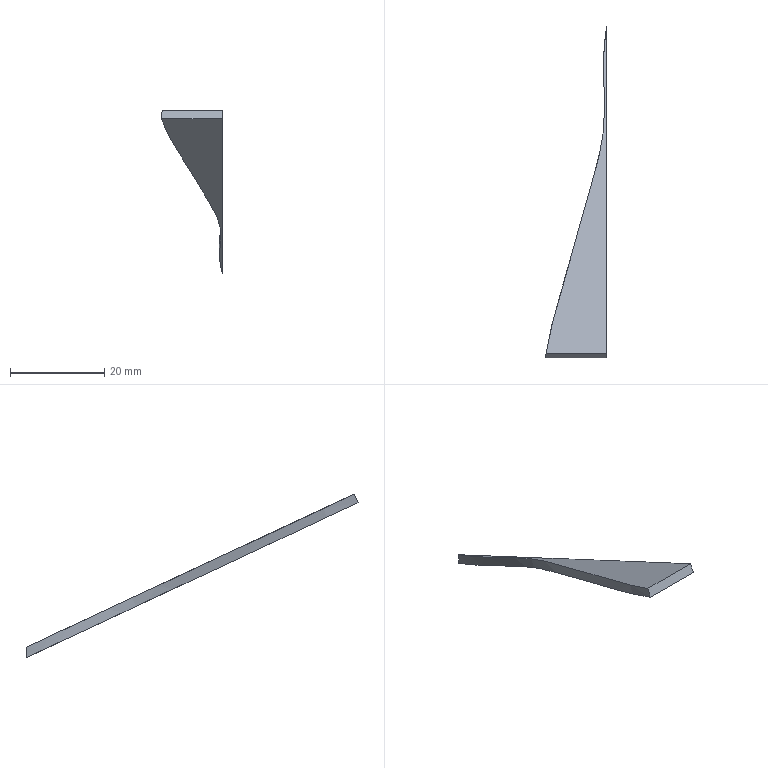Part | NX | features solid 2 | 1 solid | 5 faces | box 12.913 x 70.296 x 34.592 mm | volume 729.342 mm3 | plane 4 | spline 1
STEP:
#1=CARTESIAN_POINT('',(764.53,225.774,-99.063));
#2=VERTEX_POINT('',#1);
#3=CARTESIAN_POINT('',(777.317,295.224,-131.448));
#4=VERTEX_POINT('',#3);
#5=CARTESIAN_POINT('',(764.53,225.774,-99.063));
#6=CARTESIAN_POINT('',(764.988,228.719,-100.436));
#7=CARTESIAN_POINT('',(766.283,234.526,-103.144));
#8=CARTESIAN_POINT('',(768.978,243.072,-107.129));
#9=CARTESIAN_POINT('',(771.329,251.695,-111.15));
#10=CARTESIAN_POINT('',(773.684,260.31,-115.167));
#11=CARTESIAN_POINT('',(776.335,268.888,-119.168));
#12=CARTESIAN_POINT('',(777.182,277.623,-123.241));
#13=CARTESIAN_POINT('',(776.394,286.496,-127.378));
#14=CARTESIAN_POINT('',(776.931,292.322,-130.095));
#15=CARTESIAN_POINT('',(777.317,295.224,-131.448));
#16=B_SPLINE_CURVE_WITH_KNOTS('',3,(#5,#6,#7,#8,#9,#10,#11,#12,#13,#14,#15),.UNSPECIFIED.,.F.,.F.,(4,1,1,1,1,1,1,1,4),(0.,0.009799,0.0196,0.0294,0.0392,0.04899,0.05879,0.06859,0.07839),.UNSPECIFIED.);
#17=EDGE_CURVE('',#2,#4,#16,.T.);
#18=ORIENTED_EDGE('',*,*,#17,.F.);
#19=CARTESIAN_POINT('',(777.317,225.774,-99.063));
#20=VERTEX_POINT('',#19);
#21=CARTESIAN_POINT('',(750.,225.774,-99.063));
#22=DIRECTION('',(1.,0.,0.));
#23=VECTOR('',#22,1000.);
#24=LINE('',#21,#23);
#25=EDGE_CURVE('',#20,#2,#24,.F.);
#26=ORIENTED_EDGE('',*,*,#25,.F.);
#27=CARTESIAN_POINT('',(777.317,325.448,-145.542));
#28=DIRECTION('',(0.,-0.9063,0.4226));
#29=VECTOR('',#28,1000.);
#30=LINE('',#27,#29);
#31=EDGE_CURVE('',#4,#20,#30,.T.);
#32=ORIENTED_EDGE('',*,*,#31,.F.);
#33=EDGE_LOOP('',(#18,#26,#32));
#34=FACE_BOUND('',#33,.T.);
#35=CARTESIAN_POINT('',(750.,588.297,-268.11));
#36=DIRECTION('',(0.,0.4226,0.9063));
#37=DIRECTION('',(1.,0.,0.));
#38=AXIS2_PLACEMENT_3D('',#35,#36,#37);
#39=PLANE('',#38);
#40=ADVANCED_FACE('',(#34),#39,.T.);
#41=CARTESIAN_POINT('',(777.317,224.929,-100.876));
#42=VERTEX_POINT('',#41);
#43=CARTESIAN_POINT('',(764.403,224.929,-100.876));
#44=VERTEX_POINT('',#43);
#45=CARTESIAN_POINT('',(750.,224.929,-100.876));
#46=DIRECTION('',(1.,0.,0.));
#47=VECTOR('',#46,1000.);
#48=LINE('',#45,#47);
#49=EDGE_CURVE('',#42,#44,#48,.F.);
#50=ORIENTED_EDGE('',*,*,#49,.T.);
#51=CARTESIAN_POINT('',(777.317,295.224,-133.655));
#52=VERTEX_POINT('',#51);
#53=CARTESIAN_POINT('',(764.403,224.929,-100.876));
#54=CARTESIAN_POINT('',(764.835,227.914,-102.268));
#55=CARTESIAN_POINT('',(766.075,233.804,-105.015));
#56=CARTESIAN_POINT('',(768.784,242.455,-109.049));
#57=CARTESIAN_POINT('',(771.199,251.172,-113.113));
#58=CARTESIAN_POINT('',(773.555,259.893,-117.18));
#59=CARTESIAN_POINT('',(776.264,268.571,-121.226));
#60=CARTESIAN_POINT('',(777.189,277.406,-125.346));
#61=CARTESIAN_POINT('',(776.555,284.89,-128.836));
#62=CARTESIAN_POINT('',(776.745,290.816,-131.6));
#63=CARTESIAN_POINT('',(777.121,293.755,-132.97));
#64=CARTESIAN_POINT('',(777.317,295.224,-133.655));
#65=B_SPLINE_CURVE_WITH_KNOTS('',3,(#53,#54,#55,#56,#57,#58,#59,#60,#61,#62,#63,#64),.UNSPECIFIED.,.F.,.F.,(4,1,1,1,1,1,1,1,1,4),(0.,0.009914,0.01983,0.02974,0.03966,0.04957,0.05948,0.0694,0.07435,0.07931),.UNSPECIFIED.);
#66=EDGE_CURVE('',#44,#52,#65,.T.);
#67=ORIENTED_EDGE('',*,*,#66,.T.);
#68=CARTESIAN_POINT('',(777.317,324.603,-147.355));
#69=DIRECTION('',(0.,-0.9063,0.4226));
#70=VECTOR('',#69,1000.);
#71=LINE('',#68,#70);
#72=EDGE_CURVE('',#52,#42,#71,.T.);
#73=ORIENTED_EDGE('',*,*,#72,.T.);
#74=EDGE_LOOP('',(#50,#67,#73));
#75=FACE_BOUND('',#74,.T.);
#76=CARTESIAN_POINT('',(750.,587.452,-269.923));
#77=DIRECTION('',(0.,0.4226,0.9063));
#78=DIRECTION('',(1.,0.,0.));
#79=AXIS2_PLACEMENT_3D('',#76,#77,#78);
#80=PLANE('',#79);
#81=ADVANCED_FACE('',(#75),#80,.F.);
#82=CARTESIAN_POINT('',(764.403,224.929,-100.876));
#83=CARTESIAN_POINT('',(764.444,225.21,-100.271));
#84=CARTESIAN_POINT('',(764.486,225.492,-99.667));
#85=CARTESIAN_POINT('',(764.53,225.774,-99.063));
#86=B_SPLINE_CURVE_WITH_KNOTS('',3,(#82,#83,#84,#85),.UNSPECIFIED.,.F.,.F.,(4,4),(0.,0.002004),.UNSPECIFIED.);
#87=EDGE_CURVE('',#44,#2,#86,.T.);
#88=ORIENTED_EDGE('',*,*,#87,.F.);
#89=ORIENTED_EDGE('',*,*,#49,.F.);
#90=CARTESIAN_POINT('',(777.317,206.19,-141.061));
#91=DIRECTION('',(0.,0.4226,0.9063));
#92=VECTOR('',#91,1000.);
#93=LINE('',#90,#92);
#94=EDGE_CURVE('',#20,#42,#93,.F.);
#95=ORIENTED_EDGE('',*,*,#94,.F.);
#96=ORIENTED_EDGE('',*,*,#25,.T.);
#97=EDGE_LOOP('',(#88,#89,#95,#96));
#98=FACE_BOUND('',#97,.T.);
#99=CARTESIAN_POINT('',(750.,230.,-90.));
#100=DIRECTION('',(0.,0.9063,-0.4226));
#101=DIRECTION('',(-1.,0.,0.));
#102=AXIS2_PLACEMENT_3D('',#99,#100,#101);
#103=PLANE('',#102);
#104=ADVANCED_FACE('',(#98),#103,.F.);
#105=CARTESIAN_POINT('',(777.317,295.224,600.));
#106=DIRECTION('',(0.,0.,-1.));
#107=VECTOR('',#106,1000.);
#108=LINE('',#105,#107);
#109=EDGE_CURVE('',#4,#52,#108,.T.);
#110=ORIENTED_EDGE('',*,*,#109,.F.);
#111=ORIENTED_EDGE('',*,*,#31,.T.);
#112=ORIENTED_EDGE('',*,*,#94,.T.);
#113=ORIENTED_EDGE('',*,*,#72,.F.);
#114=EDGE_LOOP('',(#110,#111,#112,#113));
#115=FACE_BOUND('',#114,.T.);
#116=CARTESIAN_POINT('',(777.317,305.865,-187.54));
#117=DIRECTION('',(1.,0.,0.));
#118=DIRECTION('',(0.,1.,0.));
#119=AXIS2_PLACEMENT_3D('',#116,#117,#118);
#120=PLANE('',#119);
#121=ADVANCED_FACE('',(#115),#120,.T.);
#122=ORIENTED_EDGE('',*,*,#87,.T.);
#123=ORIENTED_EDGE('',*,*,#17,.T.);
#124=ORIENTED_EDGE('',*,*,#109,.T.);
#125=ORIENTED_EDGE('',*,*,#66,.F.);
#126=EDGE_LOOP('',(#122,#123,#124,#125));
#127=FACE_BOUND('',#126,.T.);
#128=CARTESIAN_POINT('',(777.317,295.224,-98.856));
#129=CARTESIAN_POINT('',(777.317,295.224,-133.863));
#130=CARTESIAN_POINT('',(777.118,293.73,-98.856));
#131=CARTESIAN_POINT('',(777.118,293.73,-133.863));
#132=CARTESIAN_POINT('',(776.735,290.738,-98.856));
#133=CARTESIAN_POINT('',(776.735,290.738,-133.863));
#134=CARTESIAN_POINT('',(776.564,284.708,-98.856));
#135=CARTESIAN_POINT('',(776.564,284.708,-133.863));
#136=CARTESIAN_POINT('',(777.055,278.679,-98.856));
#137=CARTESIAN_POINT('',(777.055,278.679,-133.863));
#138=CARTESIAN_POINT('',(776.729,272.646,-98.856));
#139=CARTESIAN_POINT('',(776.729,272.646,-133.863));
#140=CARTESIAN_POINT('',(775.682,266.716,-98.856));
#141=CARTESIAN_POINT('',(775.682,266.716,-133.863));
#142=CARTESIAN_POINT('',(773.439,259.484,-98.856));
#143=CARTESIAN_POINT('',(773.439,259.484,-133.863));
#144=CARTESIAN_POINT('',(771.094,250.759,-98.856));
#145=CARTESIAN_POINT('',(771.094,250.759,-133.863));
#146=CARTESIAN_POINT('',(768.655,242.048,-98.856));
#147=CARTESIAN_POINT('',(768.655,242.048,-133.863));
#148=CARTESIAN_POINT('',(765.964,233.402,-98.856));
#149=CARTESIAN_POINT('',(765.964,233.402,-133.863));
#150=CARTESIAN_POINT('',(764.758,227.487,-98.856));
#151=CARTESIAN_POINT('',(764.758,227.487,-133.863));
#152=CARTESIAN_POINT('',(764.343,224.501,-98.856));
#153=CARTESIAN_POINT('',(764.343,224.501,-133.863));
#154=B_SPLINE_SURFACE_WITH_KNOTS('',3,1,((#128,#129),(#130,#131),(#132,#133),(#134,#135),(#136,#137),(#138,#139),(#140,#141),(#142,#143),(#144,#145),(#146,#147),(#148,#149),(#150,#151),(#152,#153)),.SURF_OF_LINEAR_EXTRUSION.,.F.,.F.,.F.,(4,1,1,1,1,1,1,1,1,1,4),(2,2),(0.915,0.916,0.917,0.919,0.92,0.921,0.923,0.925,0.9269,0.9289,0.9309),(0.,1.),.UNSPECIFIED.);
#155=ADVANCED_FACE('',(#127),#154,.F.);
#156=CLOSED_SHELL('',(#40,#81,#104,#121,#155));
#157=MANIFOLD_SOLID_BREP('',#156);
#158=(LENGTH_UNIT()NAMED_UNIT(*)SI_UNIT(.MILLI.,.METRE.));
#159=UNCERTAINTY_MEASURE_WITH_UNIT(LENGTH_MEASURE(0.0508),#158,'','');
#160=(NAMED_UNIT(*)PLANE_ANGLE_UNIT()SI_UNIT($,.RADIAN.));
#161=(NAMED_UNIT(*)SI_UNIT($,.STERADIAN.)SOLID_ANGLE_UNIT());
#162=(GEOMETRIC_REPRESENTATION_CONTEXT(3)GLOBAL_UNCERTAINTY_ASSIGNED_CONTEXT((#159))GLOBAL_UNIT_ASSIGNED_CONTEXT((#158,#160,#161))REPRESENTATION_CONTEXT('',''));
#163=ADVANCED_BREP_SHAPE_REPRESENTATION('',(#157),#162);